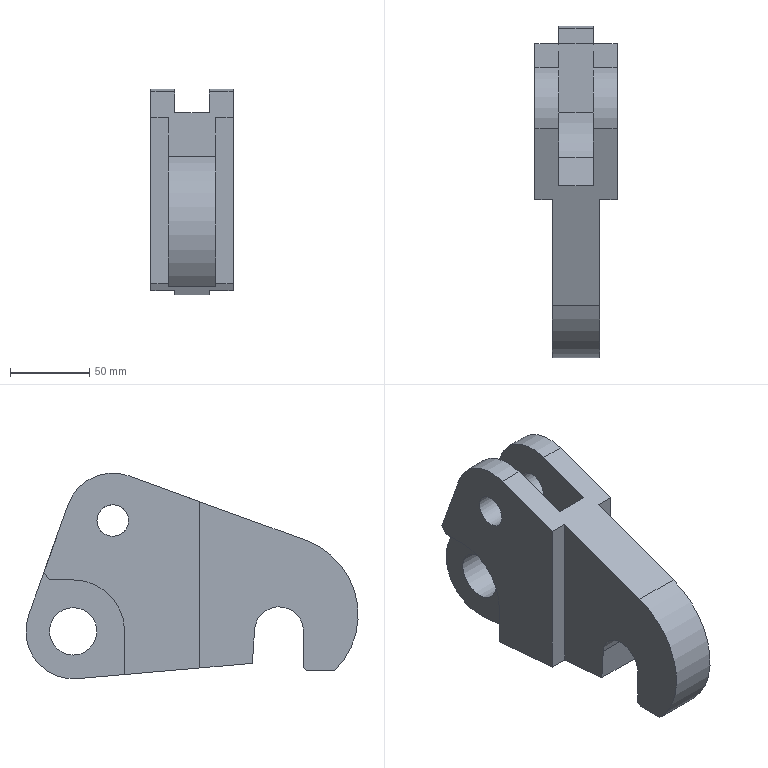Part | NX | features DATUM_CSYS 7, EXTRUDE 6, SKETCH 6, EXTRACT_FACE 2, CHAMFER 1, Instance Feature 1, Mirror Feature 1 | 1 solid | 36 faces | box 52 x 210 x 130 mm | volume 615781 mm3 | plane 25 | cylinder 11 | commonest cylinder face diameters 60 x3 65 x3 20 x2 30 x1 31 x1 100 x1
STEP:
#1=CARTESIAN_POINT('',(15.,3.252,80.09));
#2=VERTEX_POINT('',#1);
#3=CARTESIAN_POINT('',(15.,-35.261,98.191));
#4=VERTEX_POINT('',#3);
#5=CARTESIAN_POINT('',(15.,-25.,70.));
#6=DIRECTION('',(1.,0.,0.));
#7=DIRECTION('',(0.,0.,-1.));
#8=AXIS2_PLACEMENT_3D('',#5,#6,#7);
#9=CIRCLE('',#8,30.);
#10=EDGE_CURVE('',#2,#4,#9,.T.);
#11=ORIENTED_EDGE('',*,*,#10,.F.);
#12=CARTESIAN_POINT('',(0.,3.252,80.09));
#13=VERTEX_POINT('',#12);
#14=CARTESIAN_POINT('',(52.,3.252,80.09));
#15=DIRECTION('',(-1.,0.,0.));
#16=VECTOR('',#15,1000.);
#17=LINE('',#14,#16);
#18=EDGE_CURVE('',#2,#13,#17,.T.);
#19=ORIENTED_EDGE('',*,*,#18,.T.);
#20=CARTESIAN_POINT('',(0.,-35.261,98.191));
#21=VERTEX_POINT('',#20);
#22=CARTESIAN_POINT('',(0.,-25.,70.));
#23=DIRECTION('',(1.,0.,0.));
#24=DIRECTION('',(0.,1.,0.));
#25=AXIS2_PLACEMENT_3D('',#22,#23,#24);
#26=CIRCLE('',#25,30.);
#27=EDGE_CURVE('',#13,#21,#26,.T.);
#28=ORIENTED_EDGE('',*,*,#27,.T.);
#29=CARTESIAN_POINT('',(52.,-35.261,98.191));
#30=DIRECTION('',(-1.,0.,0.));
#31=VECTOR('',#30,1000.);
#32=LINE('',#29,#31);
#33=EDGE_CURVE('',#4,#21,#32,.T.);
#34=ORIENTED_EDGE('',*,*,#33,.F.);
#35=EDGE_LOOP('',(#11,#19,#28,#34));
#36=FACE_BOUND('',#35,.T.);
#37=CARTESIAN_POINT('',(52.,-25.,70.));
#38=DIRECTION('',(-1.,0.,0.));
#39=DIRECTION('',(0.,0.,1.));
#40=AXIS2_PLACEMENT_3D('',#37,#38,#39);
#41=CYLINDRICAL_SURFACE('',#40,30.);
#42=ADVANCED_FACE('',(#36),#41,.T.);
#43=CARTESIAN_POINT('',(0.,-15.,70.));
#44=VERTEX_POINT('',#43);
#45=CARTESIAN_POINT('',(0.,-25.,70.));
#46=DIRECTION('',(1.,0.,0.));
#47=DIRECTION('',(0.,1.,0.));
#48=AXIS2_PLACEMENT_3D('',#45,#46,#47);
#49=CIRCLE('',#48,10.);
#50=EDGE_CURVE('',#44,#44,#49,.T.);
#51=ORIENTED_EDGE('',*,*,#50,.F.);
#52=EDGE_LOOP('',(#51));
#53=FACE_BOUND('',#52,.T.);
#54=CARTESIAN_POINT('',(15.,-25.,60.));
#55=VERTEX_POINT('',#54);
#56=CARTESIAN_POINT('',(15.,-25.,70.));
#57=DIRECTION('',(1.,0.,0.));
#58=DIRECTION('',(0.,0.,-1.));
#59=AXIS2_PLACEMENT_3D('',#56,#57,#58);
#60=CIRCLE('',#59,10.);
#61=EDGE_CURVE('',#55,#55,#60,.T.);
#62=ORIENTED_EDGE('',*,*,#61,.T.);
#63=EDGE_LOOP('',(#62));
#64=FACE_BOUND('',#63,.T.);
#65=CARTESIAN_POINT('',(52.,-25.,70.));
#66=DIRECTION('',(-1.,0.,0.));
#67=DIRECTION('',(0.,0.,1.));
#68=AXIS2_PLACEMENT_3D('',#65,#66,#67);
#69=CYLINDRICAL_SURFACE('',#68,10.);
#70=ADVANCED_FACE('',(#53,#64),#69,.F.);
#71=CARTESIAN_POINT('',(15.,-32.5,-27.271));
#72=VERTEX_POINT('',#71);
#73=CARTESIAN_POINT('',(0.,-32.5,-27.271));
#74=VERTEX_POINT('',#73);
#75=CARTESIAN_POINT('',(52.,-32.5,-27.271));
#76=DIRECTION('',(-1.,0.,0.));
#77=VECTOR('',#76,1000.);
#78=LINE('',#75,#77);
#79=EDGE_CURVE('',#72,#74,#78,.T.);
#80=ORIENTED_EDGE('',*,*,#79,.F.);
#81=CARTESIAN_POINT('',(15.,-2.615,-29.886));
#82=VERTEX_POINT('',#81);
#83=CARTESIAN_POINT('',(15.,-15.067,-28.796));
#84=DIRECTION('',(0.,0.9962,-0.08716));
#85=VECTOR('',#84,1000.);
#86=LINE('',#83,#85);
#87=EDGE_CURVE('',#72,#82,#86,.T.);
#88=ORIENTED_EDGE('',*,*,#87,.T.);
#89=CARTESIAN_POINT('',(37.,-2.615,-29.886));
#90=VERTEX_POINT('',#89);
#91=CARTESIAN_POINT('',(52.,-2.615,-29.886));
#92=DIRECTION('',(-1.,0.,0.));
#93=VECTOR('',#92,1000.);
#94=LINE('',#91,#93);
#95=EDGE_CURVE('',#90,#82,#94,.T.);
#96=ORIENTED_EDGE('',*,*,#95,.F.);
#97=CARTESIAN_POINT('',(37.,-32.5,-27.271));
#98=VERTEX_POINT('',#97);
#99=CARTESIAN_POINT('',(37.,-15.067,-28.796));
#100=DIRECTION('',(0.,0.9962,-0.08716));
#101=VECTOR('',#100,1000.);
#102=LINE('',#99,#101);
#103=EDGE_CURVE('',#98,#90,#102,.T.);
#104=ORIENTED_EDGE('',*,*,#103,.F.);
#105=CARTESIAN_POINT('',(52.,-32.5,-27.271));
#106=VERTEX_POINT('',#105);
#107=CARTESIAN_POINT('',(52.,-32.5,-27.271));
#108=DIRECTION('',(1.,0.,0.));
#109=VECTOR('',#108,1000.);
#110=LINE('',#107,#109);
#111=EDGE_CURVE('',#98,#106,#110,.T.);
#112=ORIENTED_EDGE('',*,*,#111,.T.);
#113=CARTESIAN_POINT('',(52.,-80.,-23.116));
#114=VERTEX_POINT('',#113);
#115=CARTESIAN_POINT('',(52.,-113.209,-20.21));
#116=DIRECTION('',(0.,0.9962,-0.08716));
#117=VECTOR('',#116,1000.);
#118=LINE('',#115,#117);
#119=EDGE_CURVE('',#114,#106,#118,.T.);
#120=ORIENTED_EDGE('',*,*,#119,.F.);
#121=CARTESIAN_POINT('',(41.,-80.,-23.116));
#122=VERTEX_POINT('',#121);
#123=CARTESIAN_POINT('',(52.,-80.,-23.116));
#124=DIRECTION('',(-1.,0.,0.));
#125=VECTOR('',#124,1000.);
#126=LINE('',#123,#125);
#127=EDGE_CURVE('',#114,#122,#126,.T.);
#128=ORIENTED_EDGE('',*,*,#127,.T.);
#129=CARTESIAN_POINT('',(41.,-113.209,-20.21));
#130=VERTEX_POINT('',#129);
#131=CARTESIAN_POINT('',(41.,-15.067,-28.796));
#132=DIRECTION('',(0.,-0.9962,0.08716));
#133=VECTOR('',#132,1000.);
#134=LINE('',#131,#133);
#135=EDGE_CURVE('',#122,#130,#134,.T.);
#136=ORIENTED_EDGE('',*,*,#135,.T.);
#137=CARTESIAN_POINT('',(11.,-113.209,-20.21));
#138=VERTEX_POINT('',#137);
#139=CARTESIAN_POINT('',(52.,-113.209,-20.21));
#140=DIRECTION('',(-1.,0.,0.));
#141=VECTOR('',#140,1000.);
#142=LINE('',#139,#141);
#143=EDGE_CURVE('',#130,#138,#142,.T.);
#144=ORIENTED_EDGE('',*,*,#143,.T.);
#145=CARTESIAN_POINT('',(11.,-80.,-23.116));
#146=VERTEX_POINT('',#145);
#147=CARTESIAN_POINT('',(11.,-15.067,-28.796));
#148=DIRECTION('',(0.,-0.9962,0.08716));
#149=VECTOR('',#148,1000.);
#150=LINE('',#147,#149);
#151=EDGE_CURVE('',#146,#138,#150,.T.);
#152=ORIENTED_EDGE('',*,*,#151,.F.);
#153=CARTESIAN_POINT('',(0.,-80.,-23.116));
#154=VERTEX_POINT('',#153);
#155=CARTESIAN_POINT('',(52.,-80.,-23.116));
#156=DIRECTION('',(-1.,0.,0.));
#157=VECTOR('',#156,1000.);
#158=LINE('',#155,#157);
#159=EDGE_CURVE('',#146,#154,#158,.T.);
#160=ORIENTED_EDGE('',*,*,#159,.T.);
#161=CARTESIAN_POINT('',(0.,-15.067,-28.796));
#162=DIRECTION('',(0.,0.9962,-0.08716));
#163=VECTOR('',#162,1000.);
#164=LINE('',#161,#163);
#165=EDGE_CURVE('',#154,#74,#164,.T.);
#166=ORIENTED_EDGE('',*,*,#165,.T.);
#167=EDGE_LOOP('',(#80,#88,#96,#104,#112,#120,#128,#136,#144,#152,#160,#166));
#168=FACE_BOUND('',#167,.T.);
#169=CARTESIAN_POINT('',(52.,-15.067,-28.796));
#170=DIRECTION('',(0.,0.08716,0.9962));
#171=DIRECTION('',(0.,-0.9962,0.08716));
#172=AXIS2_PLACEMENT_3D('',#169,#170,#171);
#173=PLANE('',#172);
#174=ADVANCED_FACE('',(#168),#173,.F.);
#175=CARTESIAN_POINT('',(15.,28.252,10.09));
#176=VERTEX_POINT('',#175);
#177=CARTESIAN_POINT('',(15.,18.567,37.209));
#178=VERTEX_POINT('',#177);
#179=CARTESIAN_POINT('',(15.,20.249,32.5));
#180=DIRECTION('',(0.,-0.3363,0.9417));
#181=VECTOR('',#180,1000.);
#182=LINE('',#179,#181);
#183=EDGE_CURVE('',#176,#178,#182,.T.);
#184=ORIENTED_EDGE('',*,*,#183,.T.);
#185=CARTESIAN_POINT('',(0.,18.567,37.209));
#186=VERTEX_POINT('',#185);
#187=CARTESIAN_POINT('',(0.,18.567,37.209));
#188=DIRECTION('',(-1.,0.,0.));
#189=VECTOR('',#188,1000.);
#190=LINE('',#187,#189);
#191=EDGE_CURVE('',#178,#186,#190,.T.);
#192=ORIENTED_EDGE('',*,*,#191,.T.);
#193=CARTESIAN_POINT('',(0.,20.249,32.5));
#194=DIRECTION('',(0.,-0.3363,0.9417));
#195=VECTOR('',#194,1000.);
#196=LINE('',#193,#195);
#197=EDGE_CURVE('',#186,#13,#196,.T.);
#198=ORIENTED_EDGE('',*,*,#197,.T.);
#199=ORIENTED_EDGE('',*,*,#18,.F.);
#200=CARTESIAN_POINT('',(15.,18.463,37.5));
#201=VERTEX_POINT('',#200);
#202=CARTESIAN_POINT('',(15.,20.249,32.5));
#203=DIRECTION('',(0.,-0.3363,0.9417));
#204=VECTOR('',#203,1000.);
#205=LINE('',#202,#204);
#206=EDGE_CURVE('',#201,#2,#205,.T.);
#207=ORIENTED_EDGE('',*,*,#206,.F.);
#208=CARTESIAN_POINT('',(37.,18.463,37.5));
#209=VERTEX_POINT('',#208);
#210=CARTESIAN_POINT('',(52.,18.463,37.5));
#211=DIRECTION('',(-1.,0.,0.));
#212=VECTOR('',#211,1000.);
#213=LINE('',#210,#212);
#214=EDGE_CURVE('',#209,#201,#213,.T.);
#215=ORIENTED_EDGE('',*,*,#214,.F.);
#216=CARTESIAN_POINT('',(37.,3.252,80.09));
#217=VERTEX_POINT('',#216);
#218=CARTESIAN_POINT('',(37.,20.249,32.5));
#219=DIRECTION('',(0.,-0.3363,0.9417));
#220=VECTOR('',#219,1000.);
#221=LINE('',#218,#220);
#222=EDGE_CURVE('',#209,#217,#221,.T.);
#223=ORIENTED_EDGE('',*,*,#222,.T.);
#224=CARTESIAN_POINT('',(52.,3.252,80.09));
#225=VERTEX_POINT('',#224);
#226=CARTESIAN_POINT('',(52.,3.252,80.09));
#227=DIRECTION('',(-1.,0.,0.));
#228=VECTOR('',#227,1000.);
#229=LINE('',#226,#228);
#230=EDGE_CURVE('',#225,#217,#229,.T.);
#231=ORIENTED_EDGE('',*,*,#230,.F.);
#232=CARTESIAN_POINT('',(52.,18.567,37.209));
#233=VERTEX_POINT('',#232);
#234=CARTESIAN_POINT('',(52.,28.252,10.09));
#235=DIRECTION('',(0.,-0.3363,0.9417));
#236=VECTOR('',#235,1000.);
#237=LINE('',#234,#236);
#238=EDGE_CURVE('',#233,#225,#237,.T.);
#239=ORIENTED_EDGE('',*,*,#238,.F.);
#240=CARTESIAN_POINT('',(37.,18.567,37.209));
#241=VERTEX_POINT('',#240);
#242=CARTESIAN_POINT('',(52.,18.567,37.209));
#243=DIRECTION('',(-1.,0.,0.));
#244=VECTOR('',#243,1000.);
#245=LINE('',#242,#244);
#246=EDGE_CURVE('',#233,#241,#245,.T.);
#247=ORIENTED_EDGE('',*,*,#246,.T.);
#248=CARTESIAN_POINT('',(37.,28.252,10.09));
#249=VERTEX_POINT('',#248);
#250=CARTESIAN_POINT('',(37.,20.249,32.5));
#251=DIRECTION('',(0.,-0.3363,0.9417));
#252=VECTOR('',#251,1000.);
#253=LINE('',#250,#252);
#254=EDGE_CURVE('',#249,#241,#253,.T.);
#255=ORIENTED_EDGE('',*,*,#254,.F.);
#256=CARTESIAN_POINT('',(52.,28.252,10.09));
#257=DIRECTION('',(-1.,0.,0.));
#258=VECTOR('',#257,1000.);
#259=LINE('',#256,#258);
#260=EDGE_CURVE('',#249,#176,#259,.T.);
#261=ORIENTED_EDGE('',*,*,#260,.T.);
#262=EDGE_LOOP('',(#184,#192,#198,#199,#207,#215,#223,#231,#239,#247,#255,#261));
#263=FACE_BOUND('',#262,.T.);
#264=CARTESIAN_POINT('',(52.,20.249,32.5));
#265=DIRECTION('',(0.,-0.9417,-0.3363));
#266=DIRECTION('',(0.,0.3363,-0.9417));
#267=AXIS2_PLACEMENT_3D('',#264,#265,#266);
#268=PLANE('',#267);
#269=ADVANCED_FACE('',(#263),#268,.F.);
#270=CARTESIAN_POINT('',(52.,-15.,70.));
#271=VERTEX_POINT('',#270);
#272=CARTESIAN_POINT('',(52.,-25.,70.));
#273=DIRECTION('',(1.,0.,0.));
#274=DIRECTION('',(0.,1.,0.));
#275=AXIS2_PLACEMENT_3D('',#272,#273,#274);
#276=CIRCLE('',#275,10.);
#277=EDGE_CURVE('',#271,#271,#276,.T.);
#278=ORIENTED_EDGE('',*,*,#277,.F.);
#279=EDGE_LOOP('',(#278));
#280=FACE_BOUND('',#279,.T.);
#281=CARTESIAN_POINT('',(52.,15.249,32.5));
#282=VERTEX_POINT('',#281);
#283=CARTESIAN_POINT('',(52.,0.,32.5));
#284=VERTEX_POINT('',#283);
#285=CARTESIAN_POINT('',(52.,69.811,32.5));
#286=DIRECTION('',(0.,-1.,0.));
#287=VECTOR('',#286,1000.);
#288=LINE('',#285,#287);
#289=EDGE_CURVE('',#282,#284,#288,.T.);
#290=ORIENTED_EDGE('',*,*,#289,.F.);
#291=CARTESIAN_POINT('',(52.,18.567,37.209));
#292=DIRECTION('',(0.,-0.576,-0.8174));
#293=VECTOR('',#292,1000.);
#294=LINE('',#291,#293);
#295=EDGE_CURVE('',#282,#233,#294,.F.);
#296=ORIENTED_EDGE('',*,*,#295,.T.);
#297=ORIENTED_EDGE('',*,*,#238,.T.);
#298=CARTESIAN_POINT('',(52.,-35.261,98.191));
#299=VERTEX_POINT('',#298);
#300=CARTESIAN_POINT('',(52.,-25.,70.));
#301=DIRECTION('',(1.,0.,0.));
#302=DIRECTION('',(0.,1.,0.));
#303=AXIS2_PLACEMENT_3D('',#300,#301,#302);
#304=CIRCLE('',#303,30.);
#305=EDGE_CURVE('',#225,#299,#304,.T.);
#306=ORIENTED_EDGE('',*,*,#305,.T.);
#307=CARTESIAN_POINT('',(52.,-80.,81.907));
#308=VERTEX_POINT('',#307);
#309=CARTESIAN_POINT('',(52.,-35.261,98.191));
#310=DIRECTION('',(0.,-0.9397,-0.342));
#311=VECTOR('',#310,1000.);
#312=LINE('',#309,#311);
#313=EDGE_CURVE('',#299,#308,#312,.T.);
#314=ORIENTED_EDGE('',*,*,#313,.T.);
#315=CARTESIAN_POINT('',(52.,-80.,-135.863));
#316=DIRECTION('',(0.,0.,1.));
#317=VECTOR('',#316,1000.);
#318=LINE('',#315,#317);
#319=EDGE_CURVE('',#114,#308,#318,.T.);
#320=ORIENTED_EDGE('',*,*,#319,.F.);
#321=ORIENTED_EDGE('',*,*,#119,.T.);
#322=CARTESIAN_POINT('',(52.,-32.5,0.));
#323=VERTEX_POINT('',#322);
#324=CARTESIAN_POINT('',(52.,-32.5,0.));
#325=DIRECTION('',(0.,0.,-1.));
#326=VECTOR('',#325,1000.);
#327=LINE('',#324,#326);
#328=EDGE_CURVE('',#323,#106,#327,.T.);
#329=ORIENTED_EDGE('',*,*,#328,.F.);
#330=CARTESIAN_POINT('',(52.,0.,0.));
#331=DIRECTION('',(1.,0.,0.));
#332=DIRECTION('',(0.,1.,0.));
#333=AXIS2_PLACEMENT_3D('',#330,#331,#332);
#334=CIRCLE('',#333,32.5);
#335=EDGE_CURVE('',#284,#323,#334,.T.);
#336=ORIENTED_EDGE('',*,*,#335,.F.);
#337=EDGE_LOOP('',(#290,#296,#297,#306,#314,#320,#321,#329,#336));
#338=FACE_BOUND('',#337,.T.);
#339=CARTESIAN_POINT('',(52.,-130.,0.));
#340=DIRECTION('',(-1.,0.,0.));
#341=DIRECTION('',(0.,0.,1.));
#342=AXIS2_PLACEMENT_3D('',#339,#340,#341);
#343=PLANE('',#342);
#344=ADVANCED_FACE('',(#280,#338),#343,.F.);
#345=ORIENTED_EDGE('',*,*,#95,.T.);
#346=CARTESIAN_POINT('',(15.,0.,0.));
#347=DIRECTION('',(1.,0.,0.));
#348=DIRECTION('',(0.,0.,-1.));
#349=AXIS2_PLACEMENT_3D('',#346,#347,#348);
#350=CIRCLE('',#349,30.);
#351=EDGE_CURVE('',#82,#176,#350,.T.);
#352=ORIENTED_EDGE('',*,*,#351,.T.);
#353=ORIENTED_EDGE('',*,*,#260,.F.);
#354=CARTESIAN_POINT('',(37.,0.,0.));
#355=DIRECTION('',(1.,0.,0.));
#356=DIRECTION('',(0.,0.,-1.));
#357=AXIS2_PLACEMENT_3D('',#354,#355,#356);
#358=CIRCLE('',#357,30.);
#359=EDGE_CURVE('',#90,#249,#358,.T.);
#360=ORIENTED_EDGE('',*,*,#359,.F.);
#361=EDGE_LOOP('',(#345,#352,#353,#360));
#362=FACE_BOUND('',#361,.T.);
#363=CARTESIAN_POINT('',(52.,0.,0.));
#364=DIRECTION('',(-1.,0.,0.));
#365=DIRECTION('',(0.,0.,1.));
#366=AXIS2_PLACEMENT_3D('',#363,#364,#365);
#367=CYLINDRICAL_SURFACE('',#366,30.);
#368=ADVANCED_FACE('',(#362),#367,.T.);
#369=CARTESIAN_POINT('',(15.,0.,-15.));
#370=VERTEX_POINT('',#369);
#371=CARTESIAN_POINT('',(15.,0.,0.));
#372=DIRECTION('',(1.,0.,0.));
#373=DIRECTION('',(0.,0.,-1.));
#374=AXIS2_PLACEMENT_3D('',#371,#372,#373);
#375=CIRCLE('',#374,15.);
#376=EDGE_CURVE('',#370,#370,#375,.T.);
#377=ORIENTED_EDGE('',*,*,#376,.F.);
#378=EDGE_LOOP('',(#377));
#379=FACE_BOUND('',#378,.T.);
#380=CARTESIAN_POINT('',(37.,0.,-15.));
#381=VERTEX_POINT('',#380);
#382=CARTESIAN_POINT('',(37.,0.,0.));
#383=DIRECTION('',(1.,0.,0.));
#384=DIRECTION('',(0.,0.,-1.));
#385=AXIS2_PLACEMENT_3D('',#382,#383,#384);
#386=CIRCLE('',#385,15.);
#387=EDGE_CURVE('',#381,#381,#386,.T.);
#388=ORIENTED_EDGE('',*,*,#387,.T.);
#389=EDGE_LOOP('',(#388));
#390=FACE_BOUND('',#389,.T.);
#391=CARTESIAN_POINT('',(52.,0.,0.));
#392=DIRECTION('',(-1.,0.,0.));
#393=DIRECTION('',(0.,0.,1.));
#394=AXIS2_PLACEMENT_3D('',#391,#392,#393);
#395=CYLINDRICAL_SURFACE('',#394,15.);
#396=ADVANCED_FACE('',(#379,#390),#395,.F.);
#397=CARTESIAN_POINT('',(11.,-147.5,-25.));
#398=VERTEX_POINT('',#397);
#399=CARTESIAN_POINT('',(11.,-165.211,-25.));
#400=VERTEX_POINT('',#399);
#401=CARTESIAN_POINT('',(11.,-165.211,-25.));
#402=DIRECTION('',(0.,-1.,0.));
#403=VECTOR('',#402,1000.);
#404=LINE('',#401,#403);
#405=EDGE_CURVE('',#398,#400,#404,.T.);
#406=ORIENTED_EDGE('',*,*,#405,.F.);
#407=CARTESIAN_POINT('',(41.,-147.5,-25.));
#408=VERTEX_POINT('',#407);
#409=CARTESIAN_POINT('',(52.,-147.5,-25.));
#410=DIRECTION('',(-1.,0.,0.));
#411=VECTOR('',#410,1000.);
#412=LINE('',#409,#411);
#413=EDGE_CURVE('',#408,#398,#412,.T.);
#414=ORIENTED_EDGE('',*,*,#413,.F.);
#415=CARTESIAN_POINT('',(41.,-165.211,-25.));
#416=VERTEX_POINT('',#415);
#417=CARTESIAN_POINT('',(41.,-165.211,-25.));
#418=DIRECTION('',(0.,-1.,0.));
#419=VECTOR('',#418,1000.);
#420=LINE('',#417,#419);
#421=EDGE_CURVE('',#408,#416,#420,.T.);
#422=ORIENTED_EDGE('',*,*,#421,.T.);
#423=CARTESIAN_POINT('',(52.,-165.211,-25.));
#424=DIRECTION('',(-1.,0.,0.));
#425=VECTOR('',#424,1000.);
#426=LINE('',#423,#425);
#427=EDGE_CURVE('',#416,#400,#426,.T.);
#428=ORIENTED_EDGE('',*,*,#427,.T.);
#429=EDGE_LOOP('',(#406,#414,#422,#428));
#430=FACE_BOUND('',#429,.T.);
#431=CARTESIAN_POINT('',(52.,-165.211,-25.));
#432=DIRECTION('',(0.,0.,1.));
#433=DIRECTION('',(1.,0.,0.));
#434=AXIS2_PLACEMENT_3D('',#431,#432,#433);
#435=PLANE('',#434);
#436=ADVANCED_FACE('',(#430),#435,.F.);
#437=CARTESIAN_POINT('',(11.,-145.5,-23.));
#438=VERTEX_POINT('',#437);
#439=CARTESIAN_POINT('',(11.,-147.5,-25.));
#440=DIRECTION('',(0.,-0.7071,-0.7071));
#441=VECTOR('',#440,1000.);
#442=LINE('',#439,#441);
#443=EDGE_CURVE('',#438,#398,#442,.T.);
#444=ORIENTED_EDGE('',*,*,#443,.F.);
#445=CARTESIAN_POINT('',(41.,-145.5,-23.));
#446=VERTEX_POINT('',#445);
#447=CARTESIAN_POINT('',(52.,-145.5,-23.));
#448=DIRECTION('',(-1.,0.,0.));
#449=VECTOR('',#448,1000.);
#450=LINE('',#447,#449);
#451=EDGE_CURVE('',#446,#438,#450,.T.);
#452=ORIENTED_EDGE('',*,*,#451,.F.);
#453=CARTESIAN_POINT('',(41.,-147.5,-25.));
#454=DIRECTION('',(0.,-0.7071,-0.7071));
#455=VECTOR('',#454,1000.);
#456=LINE('',#453,#455);
#457=EDGE_CURVE('',#446,#408,#456,.T.);
#458=ORIENTED_EDGE('',*,*,#457,.T.);
#459=ORIENTED_EDGE('',*,*,#413,.T.);
#460=EDGE_LOOP('',(#444,#452,#458,#459));
#461=FACE_BOUND('',#460,.T.);
#462=CARTESIAN_POINT('',(52.,-147.5,-25.));
#463=DIRECTION('',(0.,-0.7071,0.7071));
#464=DIRECTION('',(0.,-0.7071,-0.7071));
#465=AXIS2_PLACEMENT_3D('',#462,#463,#464);
#466=PLANE('',#465);
#467=ADVANCED_FACE('',(#461),#466,.F.);
#468=CARTESIAN_POINT('',(11.,-145.5,0.));
#469=VERTEX_POINT('',#468);
#470=CARTESIAN_POINT('',(11.,-145.5,-23.));
#471=DIRECTION('',(0.,0.,-1.));
#472=VECTOR('',#471,1000.);
#473=LINE('',#470,#472);
#474=EDGE_CURVE('',#469,#438,#473,.T.);
#475=ORIENTED_EDGE('',*,*,#474,.F.);
#476=CARTESIAN_POINT('',(41.,-145.5,0.));
#477=VERTEX_POINT('',#476);
#478=CARTESIAN_POINT('',(52.,-145.5,0.));
#479=DIRECTION('',(-1.,0.,0.));
#480=VECTOR('',#479,1000.);
#481=LINE('',#478,#480);
#482=EDGE_CURVE('',#477,#469,#481,.T.);
#483=ORIENTED_EDGE('',*,*,#482,.F.);
#484=CARTESIAN_POINT('',(41.,-145.5,-23.));
#485=DIRECTION('',(0.,0.,-1.));
#486=VECTOR('',#485,1000.);
#487=LINE('',#484,#486);
#488=EDGE_CURVE('',#477,#446,#487,.T.);
#489=ORIENTED_EDGE('',*,*,#488,.T.);
#490=ORIENTED_EDGE('',*,*,#451,.T.);
#491=EDGE_LOOP('',(#475,#483,#489,#490));
#492=FACE_BOUND('',#491,.T.);
#493=CARTESIAN_POINT('',(52.,-145.5,-23.));
#494=DIRECTION('',(0.,-1.,0.));
#495=DIRECTION('',(0.,0.,-1.));
#496=AXIS2_PLACEMENT_3D('',#493,#494,#495);
#497=PLANE('',#496);
#498=ADVANCED_FACE('',(#492),#497,.F.);
#499=CARTESIAN_POINT('',(11.,-114.53,0.9651));
#500=VERTEX_POINT('',#499);
#501=CARTESIAN_POINT('',(11.,-130.,0.));
#502=DIRECTION('',(-1.,0.,0.));
#503=DIRECTION('',(0.,0.,1.));
#504=AXIS2_PLACEMENT_3D('',#501,#502,#503);
#505=CIRCLE('',#504,15.5);
#506=EDGE_CURVE('',#500,#469,#505,.F.);
#507=ORIENTED_EDGE('',*,*,#506,.F.);
#508=CARTESIAN_POINT('',(41.,-114.53,0.9651));
#509=VERTEX_POINT('',#508);
#510=CARTESIAN_POINT('',(52.,-114.53,0.9651));
#511=DIRECTION('',(-1.,0.,0.));
#512=VECTOR('',#511,1000.);
#513=LINE('',#510,#512);
#514=EDGE_CURVE('',#509,#500,#513,.T.);
#515=ORIENTED_EDGE('',*,*,#514,.F.);
#516=CARTESIAN_POINT('',(41.,-130.,0.));
#517=DIRECTION('',(-1.,0.,0.));
#518=DIRECTION('',(0.,0.,1.));
#519=AXIS2_PLACEMENT_3D('',#516,#517,#518);
#520=CIRCLE('',#519,15.5);
#521=EDGE_CURVE('',#509,#477,#520,.F.);
#522=ORIENTED_EDGE('',*,*,#521,.T.);
#523=ORIENTED_EDGE('',*,*,#482,.T.);
#524=EDGE_LOOP('',(#507,#515,#522,#523));
#525=FACE_BOUND('',#524,.T.);
#526=CARTESIAN_POINT('',(52.,-130.,0.));
#527=DIRECTION('',(-1.,0.,0.));
#528=DIRECTION('',(0.,0.,1.));
#529=AXIS2_PLACEMENT_3D('',#526,#527,#528);
#530=CYLINDRICAL_SURFACE('',#529,15.5);
#531=ADVANCED_FACE('',(#525),#530,.F.);
#532=CARTESIAN_POINT('',(11.,-114.53,0.9651));
#533=DIRECTION('',(0.,-0.06227,0.9981));
#534=VECTOR('',#533,1000.);
#535=LINE('',#532,#534);
#536=EDGE_CURVE('',#138,#500,#535,.T.);
#537=ORIENTED_EDGE('',*,*,#536,.F.);
#538=ORIENTED_EDGE('',*,*,#143,.F.);
#539=CARTESIAN_POINT('',(41.,-114.53,0.9651));
#540=DIRECTION('',(0.,-0.06227,0.9981));
#541=VECTOR('',#540,1000.);
#542=LINE('',#539,#541);
#543=EDGE_CURVE('',#130,#509,#542,.T.);
#544=ORIENTED_EDGE('',*,*,#543,.T.);
#545=ORIENTED_EDGE('',*,*,#514,.T.);
#546=EDGE_LOOP('',(#537,#538,#544,#545));
#547=FACE_BOUND('',#546,.T.);
#548=CARTESIAN_POINT('',(52.,-114.53,0.9651));
#549=DIRECTION('',(0.,0.9981,0.06227));
#550=DIRECTION('',(0.,-0.06227,0.9981));
#551=AXIS2_PLACEMENT_3D('',#548,#549,#550);
#552=PLANE('',#551);
#553=ADVANCED_FACE('',(#547),#552,.F.);
#554=CARTESIAN_POINT('',(11.,-147.101,57.484));
#555=VERTEX_POINT('',#554);
#556=CARTESIAN_POINT('',(11.,-130.,10.5));
#557=DIRECTION('',(-1.,0.,0.));
#558=DIRECTION('',(0.,0.,1.));
#559=AXIS2_PLACEMENT_3D('',#556,#557,#558);
#560=CIRCLE('',#559,50.);
#561=EDGE_CURVE('',#400,#555,#560,.T.);
#562=ORIENTED_EDGE('',*,*,#561,.F.);
#563=ORIENTED_EDGE('',*,*,#427,.F.);
#564=CARTESIAN_POINT('',(41.,-147.101,57.484));
#565=VERTEX_POINT('',#564);
#566=CARTESIAN_POINT('',(41.,-130.,10.5));
#567=DIRECTION('',(-1.,0.,0.));
#568=DIRECTION('',(0.,0.,1.));
#569=AXIS2_PLACEMENT_3D('',#566,#567,#568);
#570=CIRCLE('',#569,50.);
#571=EDGE_CURVE('',#416,#565,#570,.T.);
#572=ORIENTED_EDGE('',*,*,#571,.T.);
#573=CARTESIAN_POINT('',(52.,-147.101,57.484));
#574=DIRECTION('',(-1.,0.,0.));
#575=VECTOR('',#574,1000.);
#576=LINE('',#573,#575);
#577=EDGE_CURVE('',#565,#555,#576,.T.);
#578=ORIENTED_EDGE('',*,*,#577,.T.);
#579=EDGE_LOOP('',(#562,#563,#572,#578));
#580=FACE_BOUND('',#579,.T.);
#581=CARTESIAN_POINT('',(52.,-130.,10.5));
#582=DIRECTION('',(-1.,0.,0.));
#583=DIRECTION('',(0.,0.,1.));
#584=AXIS2_PLACEMENT_3D('',#581,#582,#583);
#585=CYLINDRICAL_SURFACE('',#584,50.);
#586=ADVANCED_FACE('',(#580),#585,.T.);
#587=ORIENTED_EDGE('',*,*,#230,.T.);
#588=CARTESIAN_POINT('',(37.,-35.261,98.191));
#589=VERTEX_POINT('',#588);
#590=CARTESIAN_POINT('',(37.,-25.,70.));
#591=DIRECTION('',(1.,0.,0.));
#592=DIRECTION('',(0.,0.,-1.));
#593=AXIS2_PLACEMENT_3D('',#590,#591,#592);
#594=CIRCLE('',#593,30.);
#595=EDGE_CURVE('',#217,#589,#594,.T.);
#596=ORIENTED_EDGE('',*,*,#595,.T.);
#597=CARTESIAN_POINT('',(52.,-35.261,98.191));
#598=DIRECTION('',(-1.,0.,0.));
#599=VECTOR('',#598,1000.);
#600=LINE('',#597,#599);
#601=EDGE_CURVE('',#299,#589,#600,.T.);
#602=ORIENTED_EDGE('',*,*,#601,.F.);
#603=ORIENTED_EDGE('',*,*,#305,.F.);
#604=EDGE_LOOP('',(#587,#596,#602,#603));
#605=FACE_BOUND('',#604,.T.);
#606=CARTESIAN_POINT('',(52.,-25.,70.));
#607=DIRECTION('',(-1.,0.,0.));
#608=DIRECTION('',(0.,0.,1.));
#609=AXIS2_PLACEMENT_3D('',#606,#607,#608);
#610=CYLINDRICAL_SURFACE('',#609,30.);
#611=ADVANCED_FACE('',(#605),#610,.T.);
#612=ORIENTED_EDGE('',*,*,#601,.T.);
#613=CARTESIAN_POINT('',(37.,-71.243,85.094));
#614=VERTEX_POINT('',#613);
#615=CARTESIAN_POINT('',(37.,-35.261,98.191));
#616=DIRECTION('',(0.,-0.9397,-0.342));
#617=VECTOR('',#616,1000.);
#618=LINE('',#615,#617);
#619=EDGE_CURVE('',#589,#614,#618,.T.);
#620=ORIENTED_EDGE('',*,*,#619,.T.);
#621=CARTESIAN_POINT('',(15.,-71.243,85.094));
#622=VERTEX_POINT('',#621);
#623=CARTESIAN_POINT('',(52.,-71.243,85.094));
#624=DIRECTION('',(1.,0.,0.));
#625=VECTOR('',#624,1000.);
#626=LINE('',#623,#625);
#627=EDGE_CURVE('',#622,#614,#626,.T.);
#628=ORIENTED_EDGE('',*,*,#627,.F.);
#629=CARTESIAN_POINT('',(15.,-35.261,98.191));
#630=DIRECTION('',(0.,-0.9397,-0.342));
#631=VECTOR('',#630,1000.);
#632=LINE('',#629,#631);
#633=EDGE_CURVE('',#4,#622,#632,.T.);
#634=ORIENTED_EDGE('',*,*,#633,.F.);
#635=ORIENTED_EDGE('',*,*,#33,.T.);
#636=CARTESIAN_POINT('',(0.,-80.,81.907));
#637=VERTEX_POINT('',#636);
#638=CARTESIAN_POINT('',(0.,-35.261,98.191));
#639=DIRECTION('',(0.,-0.9397,-0.342));
#640=VECTOR('',#639,1000.);
#641=LINE('',#638,#640);
#642=EDGE_CURVE('',#21,#637,#641,.T.);
#643=ORIENTED_EDGE('',*,*,#642,.T.);
#644=CARTESIAN_POINT('',(11.,-80.,81.907));
#645=VERTEX_POINT('',#644);
#646=CARTESIAN_POINT('',(52.,-80.,81.907));
#647=DIRECTION('',(1.,0.,0.));
#648=VECTOR('',#647,1000.);
#649=LINE('',#646,#648);
#650=EDGE_CURVE('',#637,#645,#649,.T.);
#651=ORIENTED_EDGE('',*,*,#650,.T.);
#652=CARTESIAN_POINT('',(11.,-35.261,98.191));
#653=DIRECTION('',(0.,0.9397,0.342));
#654=VECTOR('',#653,1000.);
#655=LINE('',#652,#654);
#656=EDGE_CURVE('',#555,#645,#655,.T.);
#657=ORIENTED_EDGE('',*,*,#656,.F.);
#658=ORIENTED_EDGE('',*,*,#577,.F.);
#659=CARTESIAN_POINT('',(41.,-80.,81.907));
#660=VERTEX_POINT('',#659);
#661=CARTESIAN_POINT('',(41.,-35.261,98.191));
#662=DIRECTION('',(0.,0.9397,0.342));
#663=VECTOR('',#662,1000.);
#664=LINE('',#661,#663);
#665=EDGE_CURVE('',#565,#660,#664,.T.);
#666=ORIENTED_EDGE('',*,*,#665,.T.);
#667=CARTESIAN_POINT('',(52.,-80.,81.907));
#668=DIRECTION('',(1.,0.,0.));
#669=VECTOR('',#668,1000.);
#670=LINE('',#667,#669);
#671=EDGE_CURVE('',#660,#308,#670,.T.);
#672=ORIENTED_EDGE('',*,*,#671,.T.);
#673=ORIENTED_EDGE('',*,*,#313,.F.);
#674=EDGE_LOOP('',(#612,#620,#628,#634,#635,#643,#651,#657,#658,#666,#672,#673));
#675=FACE_BOUND('',#674,.T.);
#676=CARTESIAN_POINT('',(52.,-35.261,98.191));
#677=DIRECTION('',(0.,0.342,-0.9397));
#678=DIRECTION('',(0.,0.9397,0.342));
#679=AXIS2_PLACEMENT_3D('',#676,#677,#678);
#680=PLANE('',#679);
#681=ADVANCED_FACE('',(#675),#680,.F.);
#682=CARTESIAN_POINT('',(37.,-25.,60.));
#683=VERTEX_POINT('',#682);
#684=CARTESIAN_POINT('',(37.,-25.,70.));
#685=DIRECTION('',(1.,0.,0.));
#686=DIRECTION('',(0.,0.,-1.));
#687=AXIS2_PLACEMENT_3D('',#684,#685,#686);
#688=CIRCLE('',#687,10.);
#689=EDGE_CURVE('',#683,#683,#688,.T.);
#690=ORIENTED_EDGE('',*,*,#689,.F.);
#691=EDGE_LOOP('',(#690));
#692=FACE_BOUND('',#691,.T.);
#693=ORIENTED_EDGE('',*,*,#277,.T.);
#694=EDGE_LOOP('',(#693));
#695=FACE_BOUND('',#694,.T.);
#696=CARTESIAN_POINT('',(52.,-25.,70.));
#697=DIRECTION('',(-1.,0.,0.));
#698=DIRECTION('',(0.,0.,1.));
#699=AXIS2_PLACEMENT_3D('',#696,#697,#698);
#700=CYLINDRICAL_SURFACE('',#699,10.);
#701=ADVANCED_FACE('',(#692,#695),#700,.F.);
#702=ORIENTED_EDGE('',*,*,#197,.F.);
#703=CARTESIAN_POINT('',(0.,15.249,32.5));
#704=VERTEX_POINT('',#703);
#705=CARTESIAN_POINT('',(0.,-48.253,-57.609));
#706=DIRECTION('',(0.,-0.576,-0.8174));
#707=VECTOR('',#706,1000.);
#708=LINE('',#705,#707);
#709=EDGE_CURVE('',#186,#704,#708,.T.);
#710=ORIENTED_EDGE('',*,*,#709,.T.);
#711=CARTESIAN_POINT('',(0.,0.,32.5));
#712=VERTEX_POINT('',#711);
#713=CARTESIAN_POINT('',(0.,69.811,32.5));
#714=DIRECTION('',(0.,-1.,0.));
#715=VECTOR('',#714,1000.);
#716=LINE('',#713,#715);
#717=EDGE_CURVE('',#704,#712,#716,.T.);
#718=ORIENTED_EDGE('',*,*,#717,.T.);
#719=CARTESIAN_POINT('',(0.,-32.5,0.));
#720=VERTEX_POINT('',#719);
#721=CARTESIAN_POINT('',(0.,0.,0.));
#722=DIRECTION('',(1.,0.,0.));
#723=DIRECTION('',(0.,1.,0.));
#724=AXIS2_PLACEMENT_3D('',#721,#722,#723);
#725=CIRCLE('',#724,32.5);
#726=EDGE_CURVE('',#712,#720,#725,.T.);
#727=ORIENTED_EDGE('',*,*,#726,.T.);
#728=CARTESIAN_POINT('',(0.,-32.5,0.));
#729=DIRECTION('',(0.,0.,-1.));
#730=VECTOR('',#729,1000.);
#731=LINE('',#728,#730);
#732=EDGE_CURVE('',#720,#74,#731,.T.);
#733=ORIENTED_EDGE('',*,*,#732,.T.);
#734=ORIENTED_EDGE('',*,*,#165,.F.);
#735=CARTESIAN_POINT('',(0.,-80.,135.));
#736=DIRECTION('',(0.,0.,-1.));
#737=VECTOR('',#736,1000.);
#738=LINE('',#735,#737);
#739=EDGE_CURVE('',#637,#154,#738,.T.);
#740=ORIENTED_EDGE('',*,*,#739,.F.);
#741=ORIENTED_EDGE('',*,*,#642,.F.);
#742=ORIENTED_EDGE('',*,*,#27,.F.);
#743=EDGE_LOOP('',(#702,#710,#718,#727,#733,#734,#740,#741,#742));
#744=FACE_BOUND('',#743,.T.);
#745=ORIENTED_EDGE('',*,*,#50,.T.);
#746=EDGE_LOOP('',(#745));
#747=FACE_BOUND('',#746,.T.);
#748=CARTESIAN_POINT('',(0.,-130.,0.));
#749=DIRECTION('',(-1.,0.,0.));
#750=DIRECTION('',(0.,0.,1.));
#751=AXIS2_PLACEMENT_3D('',#748,#749,#750);
#752=PLANE('',#751);
#753=ADVANCED_FACE('',(#744,#747),#752,.T.);
#754=CARTESIAN_POINT('',(41.,-80.,-135.863));
#755=DIRECTION('',(0.,0.,1.));
#756=VECTOR('',#755,1000.);
#757=LINE('',#754,#756);
#758=EDGE_CURVE('',#660,#122,#757,.F.);
#759=ORIENTED_EDGE('',*,*,#758,.F.);
#760=ORIENTED_EDGE('',*,*,#665,.F.);
#761=ORIENTED_EDGE('',*,*,#571,.F.);
#762=ORIENTED_EDGE('',*,*,#421,.F.);
#763=ORIENTED_EDGE('',*,*,#457,.F.);
#764=ORIENTED_EDGE('',*,*,#488,.F.);
#765=ORIENTED_EDGE('',*,*,#521,.F.);
#766=ORIENTED_EDGE('',*,*,#543,.F.);
#767=ORIENTED_EDGE('',*,*,#135,.F.);
#768=EDGE_LOOP('',(#759,#760,#761,#762,#763,#764,#765,#766,#767));
#769=FACE_BOUND('',#768,.T.);
#770=CARTESIAN_POINT('',(41.,0.,0.));
#771=DIRECTION('',(-1.,0.,0.));
#772=DIRECTION('',(0.,0.,1.));
#773=AXIS2_PLACEMENT_3D('',#770,#771,#772);
#774=PLANE('',#773);
#775=ADVANCED_FACE('',(#769),#774,.F.);
#776=ORIENTED_EDGE('',*,*,#319,.T.);
#777=ORIENTED_EDGE('',*,*,#671,.F.);
#778=ORIENTED_EDGE('',*,*,#758,.T.);
#779=ORIENTED_EDGE('',*,*,#127,.F.);
#780=EDGE_LOOP('',(#776,#777,#778,#779));
#781=FACE_BOUND('',#780,.T.);
#782=CARTESIAN_POINT('',(41.,-80.,-135.863));
#783=DIRECTION('',(0.,1.,0.));
#784=DIRECTION('',(0.,0.,1.));
#785=AXIS2_PLACEMENT_3D('',#782,#783,#784);
#786=PLANE('',#785);
#787=ADVANCED_FACE('',(#781),#786,.F.);
#788=ORIENTED_EDGE('',*,*,#151,.T.);
#789=ORIENTED_EDGE('',*,*,#536,.T.);
#790=ORIENTED_EDGE('',*,*,#506,.T.);
#791=ORIENTED_EDGE('',*,*,#474,.T.);
#792=ORIENTED_EDGE('',*,*,#443,.T.);
#793=ORIENTED_EDGE('',*,*,#405,.T.);
#794=ORIENTED_EDGE('',*,*,#561,.T.);
#795=ORIENTED_EDGE('',*,*,#656,.T.);
#796=CARTESIAN_POINT('',(11.,-80.,135.));
#797=DIRECTION('',(0.,0.,-1.));
#798=VECTOR('',#797,1000.);
#799=LINE('',#796,#798);
#800=EDGE_CURVE('',#146,#645,#799,.F.);
#801=ORIENTED_EDGE('',*,*,#800,.F.);
#802=EDGE_LOOP('',(#788,#789,#790,#791,#792,#793,#794,#795,#801));
#803=FACE_BOUND('',#802,.T.);
#804=CARTESIAN_POINT('',(11.,0.,0.));
#805=DIRECTION('',(-1.,0.,0.));
#806=DIRECTION('',(0.,0.,1.));
#807=AXIS2_PLACEMENT_3D('',#804,#805,#806);
#808=PLANE('',#807);
#809=ADVANCED_FACE('',(#803),#808,.T.);
#810=ORIENTED_EDGE('',*,*,#800,.T.);
#811=ORIENTED_EDGE('',*,*,#650,.F.);
#812=ORIENTED_EDGE('',*,*,#739,.T.);
#813=ORIENTED_EDGE('',*,*,#159,.F.);
#814=EDGE_LOOP('',(#810,#811,#812,#813));
#815=FACE_BOUND('',#814,.T.);
#816=CARTESIAN_POINT('',(11.,-80.,135.));
#817=DIRECTION('',(0.,1.,0.));
#818=DIRECTION('',(0.,0.,1.));
#819=AXIS2_PLACEMENT_3D('',#816,#817,#818);
#820=PLANE('',#819);
#821=ADVANCED_FACE('',(#815),#820,.F.);
#822=CARTESIAN_POINT('',(37.,-32.5,0.));
#823=VERTEX_POINT('',#822);
#824=CARTESIAN_POINT('',(37.,-32.5,0.));
#825=DIRECTION('',(0.,0.,-1.));
#826=VECTOR('',#825,1000.);
#827=LINE('',#824,#826);
#828=EDGE_CURVE('',#98,#823,#827,.F.);
#829=ORIENTED_EDGE('',*,*,#828,.T.);
#830=CARTESIAN_POINT('',(37.,-32.5,0.));
#831=DIRECTION('',(1.,0.,0.));
#832=VECTOR('',#831,1000.);
#833=LINE('',#830,#832);
#834=EDGE_CURVE('',#323,#823,#833,.F.);
#835=ORIENTED_EDGE('',*,*,#834,.F.);
#836=ORIENTED_EDGE('',*,*,#328,.T.);
#837=ORIENTED_EDGE('',*,*,#111,.F.);
#838=EDGE_LOOP('',(#829,#835,#836,#837));
#839=FACE_BOUND('',#838,.T.);
#840=CARTESIAN_POINT('',(37.,-32.5,0.));
#841=DIRECTION('',(0.,-1.,0.));
#842=DIRECTION('',(0.,0.,-1.));
#843=AXIS2_PLACEMENT_3D('',#840,#841,#842);
#844=PLANE('',#843);
#845=ADVANCED_FACE('',(#839),#844,.F.);
#846=CARTESIAN_POINT('',(37.,0.,32.5));
#847=VERTEX_POINT('',#846);
#848=CARTESIAN_POINT('',(37.,15.249,32.5));
#849=VERTEX_POINT('',#848);
#850=CARTESIAN_POINT('',(37.,69.811,32.5));
#851=DIRECTION('',(0.,-1.,0.));
#852=VECTOR('',#851,1000.);
#853=LINE('',#850,#852);
#854=EDGE_CURVE('',#847,#849,#853,.F.);
#855=ORIENTED_EDGE('',*,*,#854,.T.);
#856=CARTESIAN_POINT('',(37.,15.249,32.5));
#857=DIRECTION('',(1.,0.,0.));
#858=VECTOR('',#857,1000.);
#859=LINE('',#856,#858);
#860=EDGE_CURVE('',#849,#282,#859,.T.);
#861=ORIENTED_EDGE('',*,*,#860,.T.);
#862=ORIENTED_EDGE('',*,*,#289,.T.);
#863=CARTESIAN_POINT('',(37.,0.,32.5));
#864=DIRECTION('',(1.,0.,0.));
#865=VECTOR('',#864,1000.);
#866=LINE('',#863,#865);
#867=EDGE_CURVE('',#284,#847,#866,.F.);
#868=ORIENTED_EDGE('',*,*,#867,.T.);
#869=EDGE_LOOP('',(#855,#861,#862,#868));
#870=FACE_BOUND('',#869,.T.);
#871=CARTESIAN_POINT('',(37.,69.811,32.5));
#872=DIRECTION('',(0.,0.,1.));
#873=DIRECTION('',(1.,0.,0.));
#874=AXIS2_PLACEMENT_3D('',#871,#872,#873);
#875=PLANE('',#874);
#876=ADVANCED_FACE('',(#870),#875,.F.);
#877=ORIENTED_EDGE('',*,*,#387,.F.);
#878=EDGE_LOOP('',(#877));
#879=FACE_BOUND('',#878,.T.);
#880=ORIENTED_EDGE('',*,*,#103,.T.);
#881=ORIENTED_EDGE('',*,*,#359,.T.);
#882=ORIENTED_EDGE('',*,*,#254,.T.);
#883=CARTESIAN_POINT('',(37.,18.567,37.209));
#884=DIRECTION('',(0.,0.576,0.8174));
#885=VECTOR('',#884,1000.);
#886=LINE('',#883,#885);
#887=EDGE_CURVE('',#241,#849,#886,.F.);
#888=ORIENTED_EDGE('',*,*,#887,.T.);
#889=ORIENTED_EDGE('',*,*,#854,.F.);
#890=CARTESIAN_POINT('',(37.,0.,0.));
#891=DIRECTION('',(1.,0.,0.));
#892=DIRECTION('',(0.,1.,0.));
#893=AXIS2_PLACEMENT_3D('',#890,#891,#892);
#894=CIRCLE('',#893,32.5);
#895=EDGE_CURVE('',#823,#847,#894,.F.);
#896=ORIENTED_EDGE('',*,*,#895,.F.);
#897=ORIENTED_EDGE('',*,*,#828,.F.);
#898=EDGE_LOOP('',(#880,#881,#882,#888,#889,#896,#897));
#899=FACE_BOUND('',#898,.T.);
#900=CARTESIAN_POINT('',(37.,0.,0.));
#901=DIRECTION('',(1.,0.,0.));
#902=DIRECTION('',(0.,0.,-1.));
#903=AXIS2_PLACEMENT_3D('',#900,#901,#902);
#904=PLANE('',#903);
#905=ADVANCED_FACE('',(#879,#899),#904,.T.);
#906=ORIENTED_EDGE('',*,*,#335,.T.);
#907=ORIENTED_EDGE('',*,*,#834,.T.);
#908=ORIENTED_EDGE('',*,*,#895,.T.);
#909=ORIENTED_EDGE('',*,*,#867,.F.);
#910=EDGE_LOOP('',(#906,#907,#908,#909));
#911=FACE_BOUND('',#910,.T.);
#912=CARTESIAN_POINT('',(37.,0.,0.));
#913=DIRECTION('',(1.,0.,0.));
#914=DIRECTION('',(0.,0.,-1.));
#915=AXIS2_PLACEMENT_3D('',#912,#913,#914);
#916=CYLINDRICAL_SURFACE('',#915,32.5);
#917=ADVANCED_FACE('',(#911),#916,.F.);
#918=ORIENTED_EDGE('',*,*,#376,.T.);
#919=EDGE_LOOP('',(#918));
#920=FACE_BOUND('',#919,.T.);
#921=CARTESIAN_POINT('',(15.,-32.5,0.));
#922=VERTEX_POINT('',#921);
#923=CARTESIAN_POINT('',(15.,-32.5,0.));
#924=DIRECTION('',(0.,0.,-1.));
#925=VECTOR('',#924,1000.);
#926=LINE('',#923,#925);
#927=EDGE_CURVE('',#72,#922,#926,.F.);
#928=ORIENTED_EDGE('',*,*,#927,.T.);
#929=CARTESIAN_POINT('',(15.,0.,32.5));
#930=VERTEX_POINT('',#929);
#931=CARTESIAN_POINT('',(15.,0.,0.));
#932=DIRECTION('',(1.,0.,0.));
#933=DIRECTION('',(0.,1.,0.));
#934=AXIS2_PLACEMENT_3D('',#931,#932,#933);
#935=CIRCLE('',#934,32.5);
#936=EDGE_CURVE('',#922,#930,#935,.F.);
#937=ORIENTED_EDGE('',*,*,#936,.T.);
#938=CARTESIAN_POINT('',(15.,15.249,32.5));
#939=VERTEX_POINT('',#938);
#940=CARTESIAN_POINT('',(15.,69.811,32.5));
#941=DIRECTION('',(0.,-1.,0.));
#942=VECTOR('',#941,1000.);
#943=LINE('',#940,#942);
#944=EDGE_CURVE('',#930,#939,#943,.F.);
#945=ORIENTED_EDGE('',*,*,#944,.T.);
#946=CARTESIAN_POINT('',(15.,-5.115,3.604));
#947=DIRECTION('',(0.,0.576,0.8174));
#948=VECTOR('',#947,1000.);
#949=LINE('',#946,#948);
#950=EDGE_CURVE('',#939,#178,#949,.T.);
#951=ORIENTED_EDGE('',*,*,#950,.T.);
#952=ORIENTED_EDGE('',*,*,#183,.F.);
#953=ORIENTED_EDGE('',*,*,#351,.F.);
#954=ORIENTED_EDGE('',*,*,#87,.F.);
#955=EDGE_LOOP('',(#928,#937,#945,#951,#952,#953,#954));
#956=FACE_BOUND('',#955,.T.);
#957=CARTESIAN_POINT('',(15.,0.,0.));
#958=DIRECTION('',(1.,0.,0.));
#959=DIRECTION('',(0.,0.,-1.));
#960=AXIS2_PLACEMENT_3D('',#957,#958,#959);
#961=PLANE('',#960);
#962=ADVANCED_FACE('',(#920,#956),#961,.F.);
#963=ORIENTED_EDGE('',*,*,#79,.T.);
#964=ORIENTED_EDGE('',*,*,#732,.F.);
#965=CARTESIAN_POINT('',(15.,-32.5,0.));
#966=DIRECTION('',(-1.,0.,0.));
#967=VECTOR('',#966,1000.);
#968=LINE('',#965,#967);
#969=EDGE_CURVE('',#720,#922,#968,.F.);
#970=ORIENTED_EDGE('',*,*,#969,.T.);
#971=ORIENTED_EDGE('',*,*,#927,.F.);
#972=EDGE_LOOP('',(#963,#964,#970,#971));
#973=FACE_BOUND('',#972,.T.);
#974=CARTESIAN_POINT('',(15.,-32.5,0.));
#975=DIRECTION('',(0.,1.,0.));
#976=DIRECTION('',(0.,0.,1.));
#977=AXIS2_PLACEMENT_3D('',#974,#975,#976);
#978=PLANE('',#977);
#979=ADVANCED_FACE('',(#973),#978,.T.);
#980=ORIENTED_EDGE('',*,*,#717,.F.);
#981=CARTESIAN_POINT('',(15.,15.249,32.5));
#982=DIRECTION('',(1.,0.,0.));
#983=VECTOR('',#982,1000.);
#984=LINE('',#981,#983);
#985=EDGE_CURVE('',#704,#939,#984,.T.);
#986=ORIENTED_EDGE('',*,*,#985,.T.);
#987=ORIENTED_EDGE('',*,*,#944,.F.);
#988=CARTESIAN_POINT('',(15.,0.,32.5));
#989=DIRECTION('',(-1.,0.,0.));
#990=VECTOR('',#989,1000.);
#991=LINE('',#988,#990);
#992=EDGE_CURVE('',#712,#930,#991,.F.);
#993=ORIENTED_EDGE('',*,*,#992,.F.);
#994=EDGE_LOOP('',(#980,#986,#987,#993));
#995=FACE_BOUND('',#994,.T.);
#996=CARTESIAN_POINT('',(15.,69.811,32.5));
#997=DIRECTION('',(0.,0.,-1.));
#998=DIRECTION('',(-1.,0.,0.));
#999=AXIS2_PLACEMENT_3D('',#996,#997,#998);
#1000=PLANE('',#999);
#1001=ADVANCED_FACE('',(#995),#1000,.T.);
#1002=ORIENTED_EDGE('',*,*,#726,.F.);
#1003=ORIENTED_EDGE('',*,*,#992,.T.);
#1004=ORIENTED_EDGE('',*,*,#936,.F.);
#1005=ORIENTED_EDGE('',*,*,#969,.F.);
#1006=EDGE_LOOP('',(#1002,#1003,#1004,#1005));
#1007=FACE_BOUND('',#1006,.T.);
#1008=CARTESIAN_POINT('',(15.,0.,0.));
#1009=DIRECTION('',(-1.,0.,0.));
#1010=DIRECTION('',(0.,0.,1.));
#1011=AXIS2_PLACEMENT_3D('',#1008,#1009,#1010);
#1012=CYLINDRICAL_SURFACE('',#1011,32.5);
#1013=ADVANCED_FACE('',(#1007),#1012,.F.);
#1014=ORIENTED_EDGE('',*,*,#214,.T.);
#1015=CARTESIAN_POINT('',(15.,-25.,37.5));
#1016=VERTEX_POINT('',#1015);
#1017=CARTESIAN_POINT('',(15.,-25.,37.5));
#1018=DIRECTION('',(0.,1.,0.));
#1019=VECTOR('',#1018,1000.);
#1020=LINE('',#1017,#1019);
#1021=EDGE_CURVE('',#201,#1016,#1020,.F.);
#1022=ORIENTED_EDGE('',*,*,#1021,.T.);
#1023=CARTESIAN_POINT('',(37.,-25.,37.5));
#1024=VERTEX_POINT('',#1023);
#1025=CARTESIAN_POINT('',(37.,-25.,37.5));
#1026=DIRECTION('',(-1.,0.,0.));
#1027=VECTOR('',#1026,1000.);
#1028=LINE('',#1025,#1027);
#1029=EDGE_CURVE('',#1016,#1024,#1028,.F.);
#1030=ORIENTED_EDGE('',*,*,#1029,.T.);
#1031=CARTESIAN_POINT('',(37.,-25.,37.5));
#1032=DIRECTION('',(0.,1.,0.));
#1033=VECTOR('',#1032,1000.);
#1034=LINE('',#1031,#1033);
#1035=EDGE_CURVE('',#209,#1024,#1034,.F.);
#1036=ORIENTED_EDGE('',*,*,#1035,.F.);
#1037=EDGE_LOOP('',(#1014,#1022,#1030,#1036));
#1038=FACE_BOUND('',#1037,.T.);
#1039=CARTESIAN_POINT('',(37.,-25.,37.5));
#1040=DIRECTION('',(0.,0.,1.));
#1041=DIRECTION('',(1.,0.,0.));
#1042=AXIS2_PLACEMENT_3D('',#1039,#1040,#1041);
#1043=PLANE('',#1042);
#1044=ADVANCED_FACE('',(#1038),#1043,.T.);
#1045=ORIENTED_EDGE('',*,*,#627,.T.);
#1046=CARTESIAN_POINT('',(37.,-53.146,53.75));
#1047=VERTEX_POINT('',#1046);
#1048=CARTESIAN_POINT('',(37.,-109.004,150.5));
#1049=DIRECTION('',(0.,0.5,-0.866));
#1050=VECTOR('',#1049,1000.);
#1051=LINE('',#1048,#1050);
#1052=EDGE_CURVE('',#1047,#614,#1051,.F.);
#1053=ORIENTED_EDGE('',*,*,#1052,.F.);
#1054=CARTESIAN_POINT('',(15.,-53.146,53.75));
#1055=VERTEX_POINT('',#1054);
#1056=CARTESIAN_POINT('',(37.,-53.146,53.75));
#1057=DIRECTION('',(-1.,0.,0.));
#1058=VECTOR('',#1057,1000.);
#1059=LINE('',#1056,#1058);
#1060=EDGE_CURVE('',#1055,#1047,#1059,.F.);
#1061=ORIENTED_EDGE('',*,*,#1060,.F.);
#1062=CARTESIAN_POINT('',(15.,-109.004,150.5));
#1063=DIRECTION('',(0.,0.5,-0.866));
#1064=VECTOR('',#1063,1000.);
#1065=LINE('',#1062,#1064);
#1066=EDGE_CURVE('',#1055,#622,#1065,.F.);
#1067=ORIENTED_EDGE('',*,*,#1066,.T.);
#1068=EDGE_LOOP('',(#1045,#1053,#1061,#1067));
#1069=FACE_BOUND('',#1068,.T.);
#1070=CARTESIAN_POINT('',(37.,-109.004,150.5));
#1071=DIRECTION('',(0.,0.866,0.5));
#1072=DIRECTION('',(0.,-0.5,0.866));
#1073=AXIS2_PLACEMENT_3D('',#1070,#1071,#1072);
#1074=PLANE('',#1073);
#1075=ADVANCED_FACE('',(#1069),#1074,.T.);
#1076=ORIENTED_EDGE('',*,*,#689,.T.);
#1077=EDGE_LOOP('',(#1076));
#1078=FACE_BOUND('',#1077,.T.);
#1079=ORIENTED_EDGE('',*,*,#1035,.T.);
#1080=CARTESIAN_POINT('',(37.,-25.,70.));
#1081=DIRECTION('',(1.,0.,0.));
#1082=DIRECTION('',(0.,1.,0.));
#1083=AXIS2_PLACEMENT_3D('',#1080,#1081,#1082);
#1084=CIRCLE('',#1083,32.5);
#1085=EDGE_CURVE('',#1024,#1047,#1084,.F.);
#1086=ORIENTED_EDGE('',*,*,#1085,.T.);
#1087=ORIENTED_EDGE('',*,*,#1052,.T.);
#1088=ORIENTED_EDGE('',*,*,#619,.F.);
#1089=ORIENTED_EDGE('',*,*,#595,.F.);
#1090=ORIENTED_EDGE('',*,*,#222,.F.);
#1091=EDGE_LOOP('',(#1079,#1086,#1087,#1088,#1089,#1090));
#1092=FACE_BOUND('',#1091,.T.);
#1093=CARTESIAN_POINT('',(37.,-25.,70.));
#1094=DIRECTION('',(1.,0.,0.));
#1095=DIRECTION('',(0.,0.,-1.));
#1096=AXIS2_PLACEMENT_3D('',#1093,#1094,#1095);
#1097=PLANE('',#1096);
#1098=ADVANCED_FACE('',(#1078,#1092),#1097,.F.);
#1099=ORIENTED_EDGE('',*,*,#61,.F.);
#1100=EDGE_LOOP('',(#1099));
#1101=FACE_BOUND('',#1100,.T.);
#1102=ORIENTED_EDGE('',*,*,#206,.T.);
#1103=ORIENTED_EDGE('',*,*,#10,.T.);
#1104=ORIENTED_EDGE('',*,*,#633,.T.);
#1105=ORIENTED_EDGE('',*,*,#1066,.F.);
#1106=CARTESIAN_POINT('',(15.,-25.,70.));
#1107=DIRECTION('',(1.,0.,0.));
#1108=DIRECTION('',(0.,1.,0.));
#1109=AXIS2_PLACEMENT_3D('',#1106,#1107,#1108);
#1110=CIRCLE('',#1109,32.5);
#1111=EDGE_CURVE('',#1016,#1055,#1110,.F.);
#1112=ORIENTED_EDGE('',*,*,#1111,.F.);
#1113=ORIENTED_EDGE('',*,*,#1021,.F.);
#1114=EDGE_LOOP('',(#1102,#1103,#1104,#1105,#1112,#1113));
#1115=FACE_BOUND('',#1114,.T.);
#1116=CARTESIAN_POINT('',(15.,-25.,70.));
#1117=DIRECTION('',(1.,0.,0.));
#1118=DIRECTION('',(0.,0.,-1.));
#1119=AXIS2_PLACEMENT_3D('',#1116,#1117,#1118);
#1120=PLANE('',#1119);
#1121=ADVANCED_FACE('',(#1101,#1115),#1120,.T.);
#1122=ORIENTED_EDGE('',*,*,#1111,.T.);
#1123=ORIENTED_EDGE('',*,*,#1060,.T.);
#1124=ORIENTED_EDGE('',*,*,#1085,.F.);
#1125=ORIENTED_EDGE('',*,*,#1029,.F.);
#1126=EDGE_LOOP('',(#1122,#1123,#1124,#1125));
#1127=FACE_BOUND('',#1126,.T.);
#1128=CARTESIAN_POINT('',(37.,-25.,70.));
#1129=DIRECTION('',(-1.,0.,0.));
#1130=DIRECTION('',(0.,0.,1.));
#1131=AXIS2_PLACEMENT_3D('',#1128,#1129,#1130);
#1132=CYLINDRICAL_SURFACE('',#1131,32.5);
#1133=ADVANCED_FACE('',(#1127),#1132,.F.);
#1134=ORIENTED_EDGE('',*,*,#709,.F.);
#1135=ORIENTED_EDGE('',*,*,#191,.F.);
#1136=ORIENTED_EDGE('',*,*,#950,.F.);
#1137=ORIENTED_EDGE('',*,*,#985,.F.);
#1138=EDGE_LOOP('',(#1134,#1135,#1136,#1137));
#1139=FACE_BOUND('',#1138,.T.);
#1140=CARTESIAN_POINT('',(15.,15.249,32.5));
#1141=DIRECTION('',(0.,0.8174,-0.576));
#1142=DIRECTION('',(-1.,0.,0.));
#1143=AXIS2_PLACEMENT_3D('',#1140,#1141,#1142);
#1144=PLANE('',#1143);
#1145=ADVANCED_FACE('',(#1139),#1144,.T.);
#1146=ORIENTED_EDGE('',*,*,#295,.F.);
#1147=ORIENTED_EDGE('',*,*,#860,.F.);
#1148=ORIENTED_EDGE('',*,*,#887,.F.);
#1149=ORIENTED_EDGE('',*,*,#246,.F.);
#1150=EDGE_LOOP('',(#1146,#1147,#1148,#1149));
#1151=FACE_BOUND('',#1150,.T.);
#1152=CARTESIAN_POINT('',(52.,18.567,37.209));
#1153=DIRECTION('',(0.,-0.8174,0.576));
#1154=DIRECTION('',(-1.,0.,0.));
#1155=AXIS2_PLACEMENT_3D('',#1152,#1153,#1154);
#1156=PLANE('',#1155);
#1157=ADVANCED_FACE('',(#1151),#1156,.F.);
#1158=CLOSED_SHELL('',(#42,#70,#174,#269,#344,#368,#396,#436,#467,#498,#531,#553,#586,#611,#681,#701,#753,#775,#787,#809,#821,#845,#876,#905,#917,#962,#979,#1001,#1013,#1044,#1075,#1098,#1121,#1133,#1145,#1157));
#1159=MANIFOLD_SOLID_BREP('',#1158);
#1160=(LENGTH_UNIT()NAMED_UNIT(*)SI_UNIT(.MILLI.,.METRE.));
#1161=UNCERTAINTY_MEASURE_WITH_UNIT(LENGTH_MEASURE(0.00001),#1160,'','');
#1162=(NAMED_UNIT(*)PLANE_ANGLE_UNIT()SI_UNIT($,.RADIAN.));
#1163=(NAMED_UNIT(*)SI_UNIT($,.STERADIAN.)SOLID_ANGLE_UNIT());
#1164=(GEOMETRIC_REPRESENTATION_CONTEXT(3)GLOBAL_UNCERTAINTY_ASSIGNED_CONTEXT((#1161))GLOBAL_UNIT_ASSIGNED_CONTEXT((#1160,#1162,#1163))REPRESENTATION_CONTEXT('',''));
#1165=ADVANCED_BREP_SHAPE_REPRESENTATION('',(#1159),#1164);